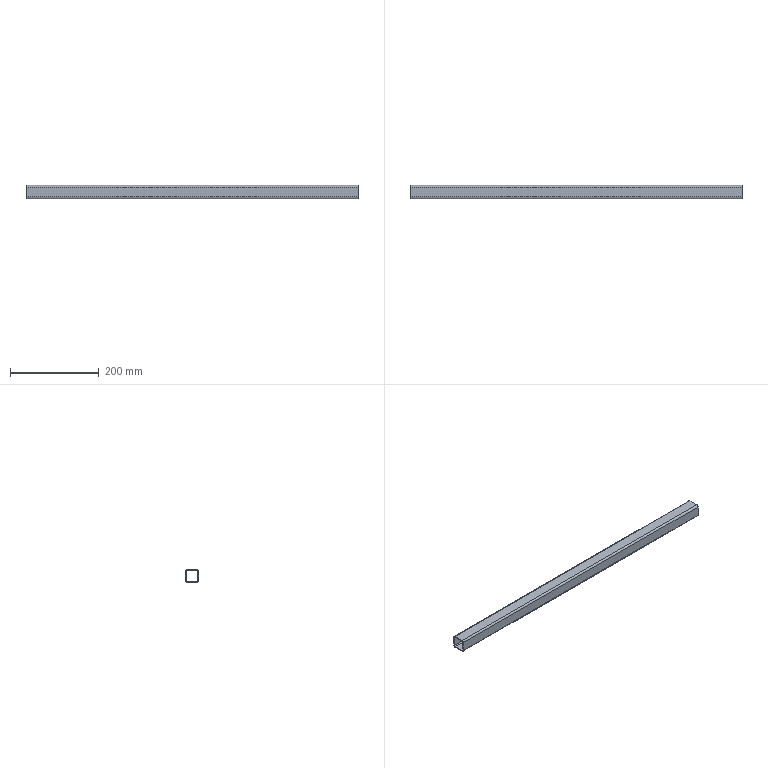Part | SolidWorks | features BaseBody 1 | 1 solid | 18 faces | box 750 x 30 x 30 mm | volume 160274 mm3 | plane 10 | cylinder 8 | commonest cylinder face diameters 4 x4 8 x4
STEP:
#1=CARTESIAN_POINT('',(-375.,-780.,407.));
#2=VERTEX_POINT('',#1);
#3=CARTESIAN_POINT('',(-375.,-776.,411.));
#4=VERTEX_POINT('',#3);
#5=CARTESIAN_POINT('',(-375.,-776.,407.));
#6=DIRECTION('',(-1.,0.,0.));
#7=DIRECTION('',(0.,0.,1.));
#8=AXIS2_PLACEMENT_3D('',#5,#6,#7);
#9=CIRCLE('',#8,4.);
#10=EDGE_CURVE('',#2,#4,#9,.T.);
#11=ORIENTED_EDGE('',*,*,#10,.F.);
#12=CARTESIAN_POINT('',(375.,-780.,407.));
#13=VERTEX_POINT('',#12);
#14=CARTESIAN_POINT('',(375.,-780.,407.));
#15=DIRECTION('',(-1.,0.,0.));
#16=VECTOR('',#15,1000.);
#17=LINE('',#14,#16);
#18=EDGE_CURVE('',#13,#2,#17,.T.);
#19=ORIENTED_EDGE('',*,*,#18,.F.);
#20=CARTESIAN_POINT('',(375.,-776.,411.));
#21=VERTEX_POINT('',#20);
#22=CARTESIAN_POINT('',(375.,-776.,407.));
#23=DIRECTION('',(1.,0.,0.));
#24=DIRECTION('',(0.,0.,-1.));
#25=AXIS2_PLACEMENT_3D('',#22,#23,#24);
#26=CIRCLE('',#25,4.);
#27=EDGE_CURVE('',#21,#13,#26,.T.);
#28=ORIENTED_EDGE('',*,*,#27,.F.);
#29=CARTESIAN_POINT('',(375.,-776.,411.));
#30=DIRECTION('',(-1.,0.,0.));
#31=VECTOR('',#30,1000.);
#32=LINE('',#29,#31);
#33=EDGE_CURVE('',#21,#4,#32,.T.);
#34=ORIENTED_EDGE('',*,*,#33,.T.);
#35=EDGE_LOOP('',(#11,#19,#28,#34));
#36=FACE_OUTER_BOUND('',#35,.T.);
#37=CARTESIAN_POINT('',(375.,-776.,407.));
#38=DIRECTION('',(-1.,0.,0.));
#39=DIRECTION('',(0.,0.,1.));
#40=AXIS2_PLACEMENT_3D('',#37,#38,#39);
#41=CYLINDRICAL_SURFACE('',#40,4.);
#42=ADVANCED_FACE('',(#36),#41,.T.);
#43=CARTESIAN_POINT('',(-375.,-780.,385.));
#44=VERTEX_POINT('',#43);
#45=CARTESIAN_POINT('',(-375.,-780.,407.));
#46=DIRECTION('',(0.,0.,1.));
#47=VECTOR('',#46,1000.);
#48=LINE('',#45,#47);
#49=EDGE_CURVE('',#44,#2,#48,.T.);
#50=ORIENTED_EDGE('',*,*,#49,.F.);
#51=CARTESIAN_POINT('',(375.,-780.,385.));
#52=VERTEX_POINT('',#51);
#53=CARTESIAN_POINT('',(375.,-780.,385.));
#54=DIRECTION('',(-1.,0.,0.));
#55=VECTOR('',#54,1000.);
#56=LINE('',#53,#55);
#57=EDGE_CURVE('',#52,#44,#56,.T.);
#58=ORIENTED_EDGE('',*,*,#57,.F.);
#59=CARTESIAN_POINT('',(375.,-780.,407.));
#60=DIRECTION('',(0.,0.,-1.));
#61=VECTOR('',#60,1000.);
#62=LINE('',#59,#61);
#63=EDGE_CURVE('',#13,#52,#62,.T.);
#64=ORIENTED_EDGE('',*,*,#63,.F.);
#65=ORIENTED_EDGE('',*,*,#18,.T.);
#66=EDGE_LOOP('',(#50,#58,#64,#65));
#67=FACE_OUTER_BOUND('',#66,.T.);
#68=CARTESIAN_POINT('',(375.,-780.,407.));
#69=DIRECTION('',(0.,1.,0.));
#70=DIRECTION('',(0.,0.,1.));
#71=AXIS2_PLACEMENT_3D('',#68,#69,#70);
#72=PLANE('',#71);
#73=ADVANCED_FACE('',(#67),#72,.F.);
#74=CARTESIAN_POINT('',(-375.,-776.,381.));
#75=VERTEX_POINT('',#74);
#76=CARTESIAN_POINT('',(-375.,-776.,385.));
#77=DIRECTION('',(-1.,0.,0.));
#78=DIRECTION('',(0.,0.,1.));
#79=AXIS2_PLACEMENT_3D('',#76,#77,#78);
#80=CIRCLE('',#79,4.);
#81=EDGE_CURVE('',#75,#44,#80,.T.);
#82=ORIENTED_EDGE('',*,*,#81,.F.);
#83=CARTESIAN_POINT('',(375.,-776.,381.));
#84=VERTEX_POINT('',#83);
#85=CARTESIAN_POINT('',(375.,-776.,381.));
#86=DIRECTION('',(-1.,0.,0.));
#87=VECTOR('',#86,1000.);
#88=LINE('',#85,#87);
#89=EDGE_CURVE('',#84,#75,#88,.T.);
#90=ORIENTED_EDGE('',*,*,#89,.F.);
#91=CARTESIAN_POINT('',(375.,-776.,385.));
#92=DIRECTION('',(1.,0.,0.));
#93=DIRECTION('',(0.,0.,-1.));
#94=AXIS2_PLACEMENT_3D('',#91,#92,#93);
#95=CIRCLE('',#94,4.);
#96=EDGE_CURVE('',#52,#84,#95,.T.);
#97=ORIENTED_EDGE('',*,*,#96,.F.);
#98=ORIENTED_EDGE('',*,*,#57,.T.);
#99=EDGE_LOOP('',(#82,#90,#97,#98));
#100=FACE_OUTER_BOUND('',#99,.T.);
#101=CARTESIAN_POINT('',(375.,-776.,385.));
#102=DIRECTION('',(-1.,0.,0.));
#103=DIRECTION('',(0.,0.,1.));
#104=AXIS2_PLACEMENT_3D('',#101,#102,#103);
#105=CYLINDRICAL_SURFACE('',#104,4.);
#106=ADVANCED_FACE('',(#100),#105,.T.);
#107=CARTESIAN_POINT('',(-375.,-754.,381.));
#108=VERTEX_POINT('',#107);
#109=CARTESIAN_POINT('',(-375.,-754.,381.));
#110=DIRECTION('',(0.,-1.,0.));
#111=VECTOR('',#110,1000.);
#112=LINE('',#109,#111);
#113=EDGE_CURVE('',#108,#75,#112,.T.);
#114=ORIENTED_EDGE('',*,*,#113,.F.);
#115=CARTESIAN_POINT('',(375.,-754.,381.));
#116=VERTEX_POINT('',#115);
#117=CARTESIAN_POINT('',(375.,-754.,381.));
#118=DIRECTION('',(-1.,0.,0.));
#119=VECTOR('',#118,1000.);
#120=LINE('',#117,#119);
#121=EDGE_CURVE('',#116,#108,#120,.T.);
#122=ORIENTED_EDGE('',*,*,#121,.F.);
#123=CARTESIAN_POINT('',(375.,-754.,381.));
#124=DIRECTION('',(0.,1.,0.));
#125=VECTOR('',#124,1000.);
#126=LINE('',#123,#125);
#127=EDGE_CURVE('',#84,#116,#126,.T.);
#128=ORIENTED_EDGE('',*,*,#127,.F.);
#129=ORIENTED_EDGE('',*,*,#89,.T.);
#130=EDGE_LOOP('',(#114,#122,#128,#129));
#131=FACE_OUTER_BOUND('',#130,.T.);
#132=CARTESIAN_POINT('',(375.,-754.,381.));
#133=DIRECTION('',(0.,0.,1.));
#134=DIRECTION('',(1.,0.,0.));
#135=AXIS2_PLACEMENT_3D('',#132,#133,#134);
#136=PLANE('',#135);
#137=ADVANCED_FACE('',(#131),#136,.F.);
#138=CARTESIAN_POINT('',(-375.,-750.,385.));
#139=VERTEX_POINT('',#138);
#140=CARTESIAN_POINT('',(-375.,-754.,385.));
#141=DIRECTION('',(-1.,0.,0.));
#142=DIRECTION('',(0.,0.,1.));
#143=AXIS2_PLACEMENT_3D('',#140,#141,#142);
#144=CIRCLE('',#143,4.);
#145=EDGE_CURVE('',#139,#108,#144,.T.);
#146=ORIENTED_EDGE('',*,*,#145,.F.);
#147=CARTESIAN_POINT('',(375.,-750.,385.));
#148=VERTEX_POINT('',#147);
#149=CARTESIAN_POINT('',(375.,-750.,385.));
#150=DIRECTION('',(-1.,0.,0.));
#151=VECTOR('',#150,1000.);
#152=LINE('',#149,#151);
#153=EDGE_CURVE('',#148,#139,#152,.T.);
#154=ORIENTED_EDGE('',*,*,#153,.F.);
#155=CARTESIAN_POINT('',(375.,-754.,385.));
#156=DIRECTION('',(1.,0.,0.));
#157=DIRECTION('',(0.,0.,-1.));
#158=AXIS2_PLACEMENT_3D('',#155,#156,#157);
#159=CIRCLE('',#158,4.);
#160=EDGE_CURVE('',#116,#148,#159,.T.);
#161=ORIENTED_EDGE('',*,*,#160,.F.);
#162=ORIENTED_EDGE('',*,*,#121,.T.);
#163=EDGE_LOOP('',(#146,#154,#161,#162));
#164=FACE_OUTER_BOUND('',#163,.T.);
#165=CARTESIAN_POINT('',(375.,-754.,385.));
#166=DIRECTION('',(-1.,0.,0.));
#167=DIRECTION('',(0.,0.,1.));
#168=AXIS2_PLACEMENT_3D('',#165,#166,#167);
#169=CYLINDRICAL_SURFACE('',#168,4.);
#170=ADVANCED_FACE('',(#164),#169,.T.);
#171=CARTESIAN_POINT('',(-375.,-750.,407.));
#172=VERTEX_POINT('',#171);
#173=CARTESIAN_POINT('',(-375.,-750.,385.));
#174=DIRECTION('',(0.,0.,-1.));
#175=VECTOR('',#174,1000.);
#176=LINE('',#173,#175);
#177=EDGE_CURVE('',#172,#139,#176,.T.);
#178=ORIENTED_EDGE('',*,*,#177,.F.);
#179=CARTESIAN_POINT('',(375.,-750.,407.));
#180=VERTEX_POINT('',#179);
#181=CARTESIAN_POINT('',(375.,-750.,407.));
#182=DIRECTION('',(-1.,0.,0.));
#183=VECTOR('',#182,1000.);
#184=LINE('',#181,#183);
#185=EDGE_CURVE('',#180,#172,#184,.T.);
#186=ORIENTED_EDGE('',*,*,#185,.F.);
#187=CARTESIAN_POINT('',(375.,-750.,385.));
#188=DIRECTION('',(0.,0.,1.));
#189=VECTOR('',#188,1000.);
#190=LINE('',#187,#189);
#191=EDGE_CURVE('',#148,#180,#190,.T.);
#192=ORIENTED_EDGE('',*,*,#191,.F.);
#193=ORIENTED_EDGE('',*,*,#153,.T.);
#194=EDGE_LOOP('',(#178,#186,#192,#193));
#195=FACE_OUTER_BOUND('',#194,.T.);
#196=CARTESIAN_POINT('',(375.,-750.,385.));
#197=DIRECTION('',(0.,-1.,0.));
#198=DIRECTION('',(0.,0.,-1.));
#199=AXIS2_PLACEMENT_3D('',#196,#197,#198);
#200=PLANE('',#199);
#201=ADVANCED_FACE('',(#195),#200,.F.);
#202=CARTESIAN_POINT('',(-375.,-754.,411.));
#203=VERTEX_POINT('',#202);
#204=CARTESIAN_POINT('',(-375.,-754.,407.));
#205=DIRECTION('',(-1.,0.,0.));
#206=DIRECTION('',(0.,0.,1.));
#207=AXIS2_PLACEMENT_3D('',#204,#205,#206);
#208=CIRCLE('',#207,4.);
#209=EDGE_CURVE('',#203,#172,#208,.T.);
#210=ORIENTED_EDGE('',*,*,#209,.F.);
#211=CARTESIAN_POINT('',(375.,-754.,411.));
#212=VERTEX_POINT('',#211);
#213=CARTESIAN_POINT('',(375.,-754.,411.));
#214=DIRECTION('',(-1.,0.,0.));
#215=VECTOR('',#214,1000.);
#216=LINE('',#213,#215);
#217=EDGE_CURVE('',#212,#203,#216,.T.);
#218=ORIENTED_EDGE('',*,*,#217,.F.);
#219=CARTESIAN_POINT('',(375.,-754.,407.));
#220=DIRECTION('',(1.,0.,0.));
#221=DIRECTION('',(0.,0.,-1.));
#222=AXIS2_PLACEMENT_3D('',#219,#220,#221);
#223=CIRCLE('',#222,4.);
#224=EDGE_CURVE('',#180,#212,#223,.T.);
#225=ORIENTED_EDGE('',*,*,#224,.F.);
#226=ORIENTED_EDGE('',*,*,#185,.T.);
#227=EDGE_LOOP('',(#210,#218,#225,#226));
#228=FACE_OUTER_BOUND('',#227,.T.);
#229=CARTESIAN_POINT('',(375.,-754.,407.));
#230=DIRECTION('',(-1.,0.,0.));
#231=DIRECTION('',(0.,0.,1.));
#232=AXIS2_PLACEMENT_3D('',#229,#230,#231);
#233=CYLINDRICAL_SURFACE('',#232,4.);
#234=ADVANCED_FACE('',(#228),#233,.T.);
#235=CARTESIAN_POINT('',(375.,-776.,383.));
#236=VERTEX_POINT('',#235);
#237=CARTESIAN_POINT('',(-375.,-776.,383.));
#238=VERTEX_POINT('',#237);
#239=CARTESIAN_POINT('',(375.,-776.,383.));
#240=DIRECTION('',(-1.,0.,0.));
#241=VECTOR('',#240,1000.);
#242=LINE('',#239,#241);
#243=EDGE_CURVE('',#236,#238,#242,.T.);
#244=ORIENTED_EDGE('',*,*,#243,.T.);
#245=CARTESIAN_POINT('',(-375.,-778.,385.));
#246=VERTEX_POINT('',#245);
#247=CARTESIAN_POINT('',(-375.,-776.,385.));
#248=DIRECTION('',(-1.,0.,0.));
#249=DIRECTION('',(0.,0.,1.));
#250=AXIS2_PLACEMENT_3D('',#247,#248,#249);
#251=CIRCLE('',#250,2.);
#252=EDGE_CURVE('',#238,#246,#251,.T.);
#253=ORIENTED_EDGE('',*,*,#252,.T.);
#254=CARTESIAN_POINT('',(375.,-778.,385.));
#255=VERTEX_POINT('',#254);
#256=CARTESIAN_POINT('',(375.,-778.,385.));
#257=DIRECTION('',(-1.,0.,0.));
#258=VECTOR('',#257,1000.);
#259=LINE('',#256,#258);
#260=EDGE_CURVE('',#255,#246,#259,.T.);
#261=ORIENTED_EDGE('',*,*,#260,.F.);
#262=CARTESIAN_POINT('',(375.,-776.,385.));
#263=DIRECTION('',(1.,0.,0.));
#264=DIRECTION('',(0.,0.,-1.));
#265=AXIS2_PLACEMENT_3D('',#262,#263,#264);
#266=CIRCLE('',#265,2.);
#267=EDGE_CURVE('',#255,#236,#266,.T.);
#268=ORIENTED_EDGE('',*,*,#267,.T.);
#269=EDGE_LOOP('',(#244,#253,#261,#268));
#270=FACE_OUTER_BOUND('',#269,.T.);
#271=CARTESIAN_POINT('',(375.,-776.,385.));
#272=DIRECTION('',(-1.,0.,0.));
#273=DIRECTION('',(0.,0.,1.));
#274=AXIS2_PLACEMENT_3D('',#271,#272,#273);
#275=CYLINDRICAL_SURFACE('',#274,2.);
#276=ADVANCED_FACE('',(#270),#275,.F.);
#277=ORIENTED_EDGE('',*,*,#260,.T.);
#278=CARTESIAN_POINT('',(-375.,-778.,407.));
#279=VERTEX_POINT('',#278);
#280=CARTESIAN_POINT('',(-375.,-778.,407.));
#281=DIRECTION('',(0.,0.,1.));
#282=VECTOR('',#281,1000.);
#283=LINE('',#280,#282);
#284=EDGE_CURVE('',#246,#279,#283,.T.);
#285=ORIENTED_EDGE('',*,*,#284,.T.);
#286=CARTESIAN_POINT('',(375.,-778.,407.));
#287=VERTEX_POINT('',#286);
#288=CARTESIAN_POINT('',(375.,-778.,407.));
#289=DIRECTION('',(-1.,0.,0.));
#290=VECTOR('',#289,1000.);
#291=LINE('',#288,#290);
#292=EDGE_CURVE('',#287,#279,#291,.T.);
#293=ORIENTED_EDGE('',*,*,#292,.F.);
#294=CARTESIAN_POINT('',(375.,-778.,407.));
#295=DIRECTION('',(0.,0.,-1.));
#296=VECTOR('',#295,1000.);
#297=LINE('',#294,#296);
#298=EDGE_CURVE('',#287,#255,#297,.T.);
#299=ORIENTED_EDGE('',*,*,#298,.T.);
#300=EDGE_LOOP('',(#277,#285,#293,#299));
#301=FACE_OUTER_BOUND('',#300,.T.);
#302=CARTESIAN_POINT('',(375.,-778.,407.));
#303=DIRECTION('',(0.,1.,0.));
#304=DIRECTION('',(0.,0.,1.));
#305=AXIS2_PLACEMENT_3D('',#302,#303,#304);
#306=PLANE('',#305);
#307=ADVANCED_FACE('',(#301),#306,.T.);
#308=ORIENTED_EDGE('',*,*,#292,.T.);
#309=CARTESIAN_POINT('',(-375.,-776.,409.));
#310=VERTEX_POINT('',#309);
#311=CARTESIAN_POINT('',(-375.,-776.,407.));
#312=DIRECTION('',(-1.,0.,0.));
#313=DIRECTION('',(0.,0.,1.));
#314=AXIS2_PLACEMENT_3D('',#311,#312,#313);
#315=CIRCLE('',#314,2.);
#316=EDGE_CURVE('',#279,#310,#315,.T.);
#317=ORIENTED_EDGE('',*,*,#316,.T.);
#318=CARTESIAN_POINT('',(375.,-776.,409.));
#319=VERTEX_POINT('',#318);
#320=CARTESIAN_POINT('',(375.,-776.,409.));
#321=DIRECTION('',(-1.,0.,0.));
#322=VECTOR('',#321,1000.);
#323=LINE('',#320,#322);
#324=EDGE_CURVE('',#319,#310,#323,.T.);
#325=ORIENTED_EDGE('',*,*,#324,.F.);
#326=CARTESIAN_POINT('',(375.,-776.,407.));
#327=DIRECTION('',(1.,0.,0.));
#328=DIRECTION('',(0.,0.,-1.));
#329=AXIS2_PLACEMENT_3D('',#326,#327,#328);
#330=CIRCLE('',#329,2.);
#331=EDGE_CURVE('',#319,#287,#330,.T.);
#332=ORIENTED_EDGE('',*,*,#331,.T.);
#333=EDGE_LOOP('',(#308,#317,#325,#332));
#334=FACE_OUTER_BOUND('',#333,.T.);
#335=CARTESIAN_POINT('',(375.,-776.,407.));
#336=DIRECTION('',(-1.,0.,0.));
#337=DIRECTION('',(0.,0.,1.));
#338=AXIS2_PLACEMENT_3D('',#335,#336,#337);
#339=CYLINDRICAL_SURFACE('',#338,2.);
#340=ADVANCED_FACE('',(#334),#339,.F.);
#341=ORIENTED_EDGE('',*,*,#324,.T.);
#342=CARTESIAN_POINT('',(-375.,-754.,409.));
#343=VERTEX_POINT('',#342);
#344=CARTESIAN_POINT('',(-375.,-776.,409.));
#345=DIRECTION('',(0.,1.,0.));
#346=VECTOR('',#345,1000.);
#347=LINE('',#344,#346);
#348=EDGE_CURVE('',#310,#343,#347,.T.);
#349=ORIENTED_EDGE('',*,*,#348,.T.);
#350=CARTESIAN_POINT('',(375.,-754.,409.));
#351=VERTEX_POINT('',#350);
#352=CARTESIAN_POINT('',(375.,-754.,409.));
#353=DIRECTION('',(-1.,0.,0.));
#354=VECTOR('',#353,1000.);
#355=LINE('',#352,#354);
#356=EDGE_CURVE('',#351,#343,#355,.T.);
#357=ORIENTED_EDGE('',*,*,#356,.F.);
#358=CARTESIAN_POINT('',(375.,-776.,409.));
#359=DIRECTION('',(0.,-1.,0.));
#360=VECTOR('',#359,1000.);
#361=LINE('',#358,#360);
#362=EDGE_CURVE('',#351,#319,#361,.T.);
#363=ORIENTED_EDGE('',*,*,#362,.T.);
#364=EDGE_LOOP('',(#341,#349,#357,#363));
#365=FACE_OUTER_BOUND('',#364,.T.);
#366=CARTESIAN_POINT('',(375.,-776.,409.));
#367=DIRECTION('',(0.,0.,-1.));
#368=DIRECTION('',(-1.,0.,0.));
#369=AXIS2_PLACEMENT_3D('',#366,#367,#368);
#370=PLANE('',#369);
#371=ADVANCED_FACE('',(#365),#370,.T.);
#372=ORIENTED_EDGE('',*,*,#356,.T.);
#373=CARTESIAN_POINT('',(-375.,-752.,407.));
#374=VERTEX_POINT('',#373);
#375=CARTESIAN_POINT('',(-375.,-754.,407.));
#376=DIRECTION('',(-1.,0.,0.));
#377=DIRECTION('',(0.,0.,1.));
#378=AXIS2_PLACEMENT_3D('',#375,#376,#377);
#379=CIRCLE('',#378,2.);
#380=EDGE_CURVE('',#343,#374,#379,.T.);
#381=ORIENTED_EDGE('',*,*,#380,.T.);
#382=CARTESIAN_POINT('',(375.,-752.,407.));
#383=VERTEX_POINT('',#382);
#384=CARTESIAN_POINT('',(375.,-752.,407.));
#385=DIRECTION('',(-1.,0.,0.));
#386=VECTOR('',#385,1000.);
#387=LINE('',#384,#386);
#388=EDGE_CURVE('',#383,#374,#387,.T.);
#389=ORIENTED_EDGE('',*,*,#388,.F.);
#390=CARTESIAN_POINT('',(375.,-754.,407.));
#391=DIRECTION('',(1.,0.,0.));
#392=DIRECTION('',(0.,0.,-1.));
#393=AXIS2_PLACEMENT_3D('',#390,#391,#392);
#394=CIRCLE('',#393,2.);
#395=EDGE_CURVE('',#383,#351,#394,.T.);
#396=ORIENTED_EDGE('',*,*,#395,.T.);
#397=EDGE_LOOP('',(#372,#381,#389,#396));
#398=FACE_OUTER_BOUND('',#397,.T.);
#399=CARTESIAN_POINT('',(375.,-754.,407.));
#400=DIRECTION('',(-1.,0.,0.));
#401=DIRECTION('',(0.,0.,1.));
#402=AXIS2_PLACEMENT_3D('',#399,#400,#401);
#403=CYLINDRICAL_SURFACE('',#402,2.);
#404=ADVANCED_FACE('',(#398),#403,.F.);
#405=ORIENTED_EDGE('',*,*,#388,.T.);
#406=CARTESIAN_POINT('',(-375.,-752.,385.));
#407=VERTEX_POINT('',#406);
#408=CARTESIAN_POINT('',(-375.,-752.,385.));
#409=DIRECTION('',(0.,0.,-1.));
#410=VECTOR('',#409,1000.);
#411=LINE('',#408,#410);
#412=EDGE_CURVE('',#374,#407,#411,.T.);
#413=ORIENTED_EDGE('',*,*,#412,.T.);
#414=CARTESIAN_POINT('',(375.,-752.,385.));
#415=VERTEX_POINT('',#414);
#416=CARTESIAN_POINT('',(375.,-752.,385.));
#417=DIRECTION('',(-1.,0.,0.));
#418=VECTOR('',#417,1000.);
#419=LINE('',#416,#418);
#420=EDGE_CURVE('',#415,#407,#419,.T.);
#421=ORIENTED_EDGE('',*,*,#420,.F.);
#422=CARTESIAN_POINT('',(375.,-752.,385.));
#423=DIRECTION('',(0.,0.,1.));
#424=VECTOR('',#423,1000.);
#425=LINE('',#422,#424);
#426=EDGE_CURVE('',#415,#383,#425,.T.);
#427=ORIENTED_EDGE('',*,*,#426,.T.);
#428=EDGE_LOOP('',(#405,#413,#421,#427));
#429=FACE_OUTER_BOUND('',#428,.T.);
#430=CARTESIAN_POINT('',(375.,-752.,385.));
#431=DIRECTION('',(0.,-1.,0.));
#432=DIRECTION('',(0.,0.,-1.));
#433=AXIS2_PLACEMENT_3D('',#430,#431,#432);
#434=PLANE('',#433);
#435=ADVANCED_FACE('',(#429),#434,.T.);
#436=ORIENTED_EDGE('',*,*,#420,.T.);
#437=CARTESIAN_POINT('',(-375.,-754.,383.));
#438=VERTEX_POINT('',#437);
#439=CARTESIAN_POINT('',(-375.,-754.,385.));
#440=DIRECTION('',(-1.,0.,0.));
#441=DIRECTION('',(0.,0.,1.));
#442=AXIS2_PLACEMENT_3D('',#439,#440,#441);
#443=CIRCLE('',#442,2.);
#444=EDGE_CURVE('',#407,#438,#443,.T.);
#445=ORIENTED_EDGE('',*,*,#444,.T.);
#446=CARTESIAN_POINT('',(375.,-754.,383.));
#447=VERTEX_POINT('',#446);
#448=CARTESIAN_POINT('',(375.,-754.,383.));
#449=DIRECTION('',(-1.,0.,0.));
#450=VECTOR('',#449,1000.);
#451=LINE('',#448,#450);
#452=EDGE_CURVE('',#447,#438,#451,.T.);
#453=ORIENTED_EDGE('',*,*,#452,.F.);
#454=CARTESIAN_POINT('',(375.,-754.,385.));
#455=DIRECTION('',(1.,0.,0.));
#456=DIRECTION('',(0.,0.,-1.));
#457=AXIS2_PLACEMENT_3D('',#454,#455,#456);
#458=CIRCLE('',#457,2.);
#459=EDGE_CURVE('',#447,#415,#458,.T.);
#460=ORIENTED_EDGE('',*,*,#459,.T.);
#461=EDGE_LOOP('',(#436,#445,#453,#460));
#462=FACE_OUTER_BOUND('',#461,.T.);
#463=CARTESIAN_POINT('',(375.,-754.,385.));
#464=DIRECTION('',(-1.,0.,0.));
#465=DIRECTION('',(0.,0.,1.));
#466=AXIS2_PLACEMENT_3D('',#463,#464,#465);
#467=CYLINDRICAL_SURFACE('',#466,2.);
#468=ADVANCED_FACE('',(#462),#467,.F.);
#469=ORIENTED_EDGE('',*,*,#452,.T.);
#470=CARTESIAN_POINT('',(-375.,-754.,383.));
#471=DIRECTION('',(0.,-1.,0.));
#472=VECTOR('',#471,1000.);
#473=LINE('',#470,#472);
#474=EDGE_CURVE('',#438,#238,#473,.T.);
#475=ORIENTED_EDGE('',*,*,#474,.T.);
#476=ORIENTED_EDGE('',*,*,#243,.F.);
#477=CARTESIAN_POINT('',(375.,-754.,383.));
#478=DIRECTION('',(0.,1.,0.));
#479=VECTOR('',#478,1000.);
#480=LINE('',#477,#479);
#481=EDGE_CURVE('',#236,#447,#480,.T.);
#482=ORIENTED_EDGE('',*,*,#481,.T.);
#483=EDGE_LOOP('',(#469,#475,#476,#482));
#484=FACE_OUTER_BOUND('',#483,.T.);
#485=CARTESIAN_POINT('',(375.,-754.,383.));
#486=DIRECTION('',(0.,0.,1.));
#487=DIRECTION('',(1.,0.,0.));
#488=AXIS2_PLACEMENT_3D('',#485,#486,#487);
#489=PLANE('',#488);
#490=ADVANCED_FACE('',(#484),#489,.T.);
#491=CARTESIAN_POINT('',(-375.,-776.,411.));
#492=DIRECTION('',(0.,1.,0.));
#493=VECTOR('',#492,1000.);
#494=LINE('',#491,#493);
#495=EDGE_CURVE('',#4,#203,#494,.T.);
#496=ORIENTED_EDGE('',*,*,#495,.F.);
#497=ORIENTED_EDGE('',*,*,#33,.F.);
#498=CARTESIAN_POINT('',(375.,-776.,411.));
#499=DIRECTION('',(0.,-1.,0.));
#500=VECTOR('',#499,1000.);
#501=LINE('',#498,#500);
#502=EDGE_CURVE('',#212,#21,#501,.T.);
#503=ORIENTED_EDGE('',*,*,#502,.F.);
#504=ORIENTED_EDGE('',*,*,#217,.T.);
#505=EDGE_LOOP('',(#496,#497,#503,#504));
#506=FACE_OUTER_BOUND('',#505,.T.);
#507=CARTESIAN_POINT('',(375.,-776.,411.));
#508=DIRECTION('',(0.,0.,-1.));
#509=DIRECTION('',(-1.,0.,0.));
#510=AXIS2_PLACEMENT_3D('',#507,#508,#509);
#511=PLANE('',#510);
#512=ADVANCED_FACE('',(#506),#511,.F.);
#513=ORIENTED_EDGE('',*,*,#267,.F.);
#514=ORIENTED_EDGE('',*,*,#298,.F.);
#515=ORIENTED_EDGE('',*,*,#331,.F.);
#516=ORIENTED_EDGE('',*,*,#362,.F.);
#517=ORIENTED_EDGE('',*,*,#395,.F.);
#518=ORIENTED_EDGE('',*,*,#426,.F.);
#519=ORIENTED_EDGE('',*,*,#459,.F.);
#520=ORIENTED_EDGE('',*,*,#481,.F.);
#521=EDGE_LOOP('',(#513,#514,#515,#516,#517,#518,#519,#520));
#522=FACE_BOUND('',#521,.T.);
#523=ORIENTED_EDGE('',*,*,#502,.T.);
#524=ORIENTED_EDGE('',*,*,#27,.T.);
#525=ORIENTED_EDGE('',*,*,#63,.T.);
#526=ORIENTED_EDGE('',*,*,#96,.T.);
#527=ORIENTED_EDGE('',*,*,#127,.T.);
#528=ORIENTED_EDGE('',*,*,#160,.T.);
#529=ORIENTED_EDGE('',*,*,#191,.T.);
#530=ORIENTED_EDGE('',*,*,#224,.T.);
#531=EDGE_LOOP('',(#523,#524,#525,#526,#527,#528,#529,#530));
#532=FACE_OUTER_BOUND('',#531,.T.);
#533=CARTESIAN_POINT('',(375.,-750.,411.));
#534=DIRECTION('',(1.,0.,0.));
#535=DIRECTION('',(0.,0.,-1.));
#536=AXIS2_PLACEMENT_3D('',#533,#534,#535);
#537=PLANE('',#536);
#538=ADVANCED_FACE('',(#522,#532),#537,.T.);
#539=ORIENTED_EDGE('',*,*,#252,.F.);
#540=ORIENTED_EDGE('',*,*,#474,.F.);
#541=ORIENTED_EDGE('',*,*,#444,.F.);
#542=ORIENTED_EDGE('',*,*,#412,.F.);
#543=ORIENTED_EDGE('',*,*,#380,.F.);
#544=ORIENTED_EDGE('',*,*,#348,.F.);
#545=ORIENTED_EDGE('',*,*,#316,.F.);
#546=ORIENTED_EDGE('',*,*,#284,.F.);
#547=EDGE_LOOP('',(#539,#540,#541,#542,#543,#544,#545,#546));
#548=FACE_BOUND('',#547,.T.);
#549=ORIENTED_EDGE('',*,*,#49,.T.);
#550=ORIENTED_EDGE('',*,*,#10,.T.);
#551=ORIENTED_EDGE('',*,*,#495,.T.);
#552=ORIENTED_EDGE('',*,*,#209,.T.);
#553=ORIENTED_EDGE('',*,*,#177,.T.);
#554=ORIENTED_EDGE('',*,*,#145,.T.);
#555=ORIENTED_EDGE('',*,*,#113,.T.);
#556=ORIENTED_EDGE('',*,*,#81,.T.);
#557=EDGE_LOOP('',(#549,#550,#551,#552,#553,#554,#555,#556));
#558=FACE_OUTER_BOUND('',#557,.T.);
#559=CARTESIAN_POINT('',(-375.,-780.,411.));
#560=DIRECTION('',(-1.,0.,0.));
#561=DIRECTION('',(0.,0.,1.));
#562=AXIS2_PLACEMENT_3D('',#559,#560,#561);
#563=PLANE('',#562);
#564=ADVANCED_FACE('',(#548,#558),#563,.T.);
#565=CLOSED_SHELL('',(#42,#73,#106,#137,#170,#201,#234,#276,#307,#340,#371,#404,#435,#468,#490,#512,#538,#564));
#566=MANIFOLD_SOLID_BREP('',#565);
#567=CARTESIAN_POINT('',(0.,0.,0.));
#568=DIRECTION('',(0.,0.,1.));
#569=DIRECTION('',(1.,0.,0.));
#570=AXIS2_PLACEMENT_3D('',#567,#568,#569);
#571=(LENGTH_UNIT()NAMED_UNIT(*)SI_UNIT(.MILLI.,.METRE.));
#572=UNCERTAINTY_MEASURE_WITH_UNIT(LENGTH_MEASURE(0.00001),#571,'','');
#573=(NAMED_UNIT(*)PLANE_ANGLE_UNIT()SI_UNIT($,.RADIAN.));
#574=(NAMED_UNIT(*)SI_UNIT($,.STERADIAN.)SOLID_ANGLE_UNIT());
#575=(GEOMETRIC_REPRESENTATION_CONTEXT(3)GLOBAL_UNCERTAINTY_ASSIGNED_CONTEXT((#572))GLOBAL_UNIT_ASSIGNED_CONTEXT((#571,#573,#574))REPRESENTATION_CONTEXT('',''));
#576=ADVANCED_BREP_SHAPE_REPRESENTATION('',(#566,#570),#575);